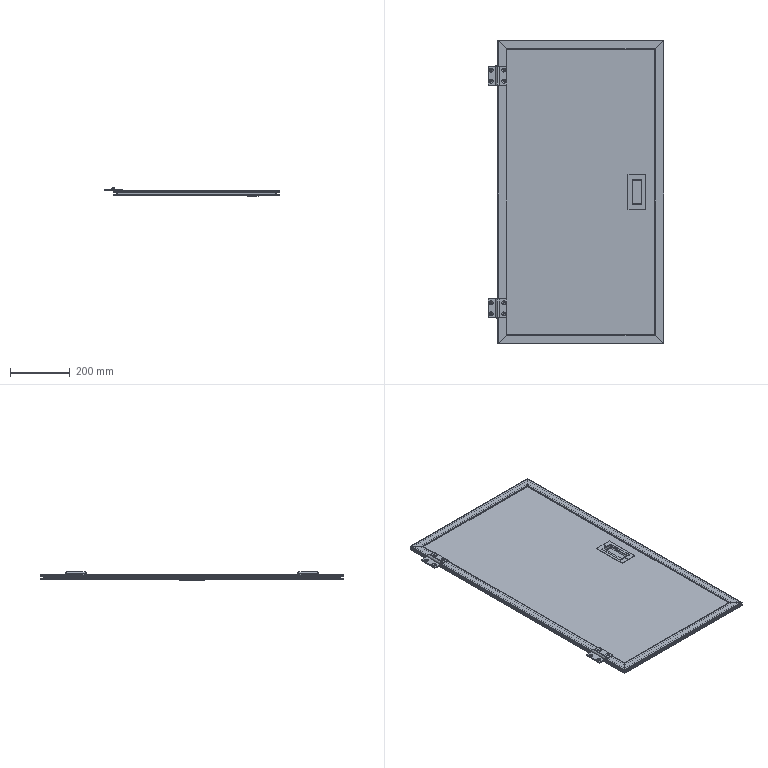Part | SolidWorks | features MoveCopyBody 3, Stock 3, ICE 2, HoleWzd 1, WeldMemberFeat 1, WeldmentFeature 1 | 8 solids | 319 faces | box 588 x 1016 x 28.7 mm | volume 3776300 mm3 | plane 165 | cylinder 110 | cone 36 | sphere 8 | commonest cylinder face diameters 5 x28 2 x20 10 x16 4 x12 15 x10 6.4 x8